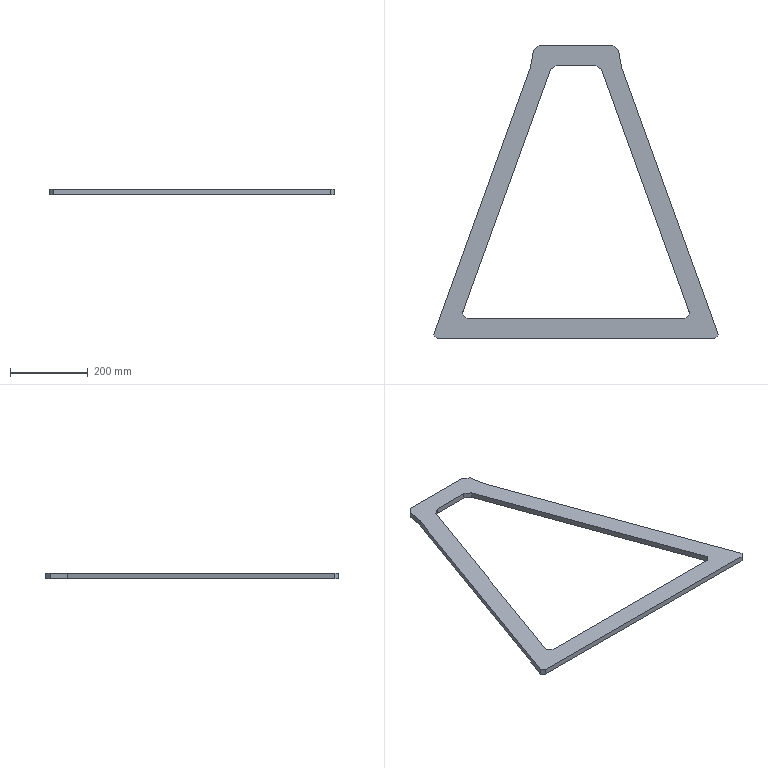Part | SolidWorks | features Extrusion 1 | 1 solid | 20 faces | box 733.425 x 755.65 x 14 mm | volume 1663233 mm3 | plane 20
STEP:
#1=CARTESIAN_POINT('',(-280.465,50.8,0.));
#2=VERTEX_POINT('',#1);
#3=CARTESIAN_POINT('',(280.465,50.8,0.));
#4=VERTEX_POINT('',#3);
#5=CARTESIAN_POINT('',(0.,50.8,0.));
#6=DIRECTION('',(1.,0.,0.));
#7=VECTOR('',#6,1000.);
#8=LINE('',#5,#7);
#9=EDGE_CURVE('',#2,#4,#8,.T.);
#10=ORIENTED_EDGE('',*,*,#9,.F.);
#11=CARTESIAN_POINT('',(-280.465,50.8,14.));
#12=VERTEX_POINT('',#11);
#13=CARTESIAN_POINT('',(-280.465,50.8,14.));
#14=DIRECTION('',(0.,0.,-1.));
#15=VECTOR('',#14,1000.);
#16=LINE('',#13,#15);
#17=EDGE_CURVE('',#12,#2,#16,.T.);
#18=ORIENTED_EDGE('',*,*,#17,.F.);
#19=CARTESIAN_POINT('',(280.465,50.8,14.));
#20=VERTEX_POINT('',#19);
#21=CARTESIAN_POINT('',(0.,50.8,14.));
#22=DIRECTION('',(1.,0.,0.));
#23=VECTOR('',#22,1000.);
#24=LINE('',#21,#23);
#25=EDGE_CURVE('',#12,#20,#24,.T.);
#26=ORIENTED_EDGE('',*,*,#25,.T.);
#27=CARTESIAN_POINT('',(280.465,50.8,14.));
#28=DIRECTION('',(0.,0.,-1.));
#29=VECTOR('',#28,1000.);
#30=LINE('',#27,#29);
#31=EDGE_CURVE('',#20,#4,#30,.T.);
#32=ORIENTED_EDGE('',*,*,#31,.T.);
#33=EDGE_LOOP('',(#10,#18,#26,#32));
#34=FACE_OUTER_BOUND('',#33,.T.);
#35=CARTESIAN_POINT('',(0.,50.8,14.));
#36=DIRECTION('',(0.,1.,0.));
#37=DIRECTION('',(0.,0.,1.));
#38=AXIS2_PLACEMENT_3D('',#35,#36,#37);
#39=PLANE('',#38);
#40=ADVANCED_FACE('',(#34),#39,.T.);
#41=CARTESIAN_POINT('',(-293.165,63.5,0.));
#42=VERTEX_POINT('',#41);
#43=CARTESIAN_POINT('',(-114.833,-114.833,0.));
#44=DIRECTION('',(-0.7071,0.7071,0.));
#45=VECTOR('',#44,1000.);
#46=LINE('',#43,#45);
#47=EDGE_CURVE('',#2,#42,#46,.T.);
#48=ORIENTED_EDGE('',*,*,#47,.T.);
#49=CARTESIAN_POINT('',(-293.165,63.5,14.));
#50=VERTEX_POINT('',#49);
#51=CARTESIAN_POINT('',(-293.165,63.5,14.));
#52=DIRECTION('',(0.,0.,-1.));
#53=VECTOR('',#52,1000.);
#54=LINE('',#51,#53);
#55=EDGE_CURVE('',#50,#42,#54,.T.);
#56=ORIENTED_EDGE('',*,*,#55,.F.);
#57=CARTESIAN_POINT('',(-114.833,-114.833,14.));
#58=DIRECTION('',(-0.7071,0.7071,0.));
#59=VECTOR('',#58,1000.);
#60=LINE('',#57,#59);
#61=EDGE_CURVE('',#12,#50,#60,.T.);
#62=ORIENTED_EDGE('',*,*,#61,.F.);
#63=ORIENTED_EDGE('',*,*,#17,.T.);
#64=EDGE_LOOP('',(#48,#56,#62,#63));
#65=FACE_OUTER_BOUND('',#64,.T.);
#66=CARTESIAN_POINT('',(-114.833,-114.833,14.));
#67=DIRECTION('',(-0.7071,-0.7071,0.));
#68=DIRECTION('',(0.7071,-0.7071,0.));
#69=AXIS2_PLACEMENT_3D('',#66,#67,#68);
#70=PLANE('',#69);
#71=ADVANCED_FACE('',(#65),#70,.F.);
#72=CARTESIAN_POINT('',(-65.476,692.907,0.));
#73=VERTEX_POINT('',#72);
#74=CARTESIAN_POINT('',(-279.553,101.129,0.));
#75=DIRECTION('',(0.3402,0.9404,0.));
#76=VECTOR('',#75,1000.);
#77=LINE('',#74,#76);
#78=EDGE_CURVE('',#42,#73,#77,.T.);
#79=ORIENTED_EDGE('',*,*,#78,.T.);
#80=CARTESIAN_POINT('',(-65.476,692.907,14.));
#81=VERTEX_POINT('',#80);
#82=CARTESIAN_POINT('',(-65.476,692.907,14.));
#83=DIRECTION('',(0.,0.,-1.));
#84=VECTOR('',#83,1000.);
#85=LINE('',#82,#84);
#86=EDGE_CURVE('',#81,#73,#85,.T.);
#87=ORIENTED_EDGE('',*,*,#86,.F.);
#88=CARTESIAN_POINT('',(-279.553,101.129,14.));
#89=DIRECTION('',(0.3402,0.9404,0.));
#90=VECTOR('',#89,1000.);
#91=LINE('',#88,#90);
#92=EDGE_CURVE('',#50,#81,#91,.T.);
#93=ORIENTED_EDGE('',*,*,#92,.F.);
#94=ORIENTED_EDGE('',*,*,#55,.T.);
#95=EDGE_LOOP('',(#79,#87,#93,#94));
#96=FACE_OUTER_BOUND('',#95,.T.);
#97=CARTESIAN_POINT('',(-279.553,101.129,14.));
#98=DIRECTION('',(-0.9404,0.3402,0.));
#99=DIRECTION('',(-0.3402,-0.9404,0.));
#100=AXIS2_PLACEMENT_3D('',#97,#98,#99);
#101=PLANE('',#100);
#102=ADVANCED_FACE('',(#96),#101,.F.);
#103=CARTESIAN_POINT('',(-48.456,704.85,0.));
#104=VERTEX_POINT('',#103);
#105=CARTESIAN_POINT('',(-347.393,495.095,0.));
#106=DIRECTION('',(0.8186,0.5744,0.));
#107=VECTOR('',#106,1000.);
#108=LINE('',#105,#107);
#109=EDGE_CURVE('',#73,#104,#108,.T.);
#110=ORIENTED_EDGE('',*,*,#109,.T.);
#111=CARTESIAN_POINT('',(-48.456,704.85,14.));
#112=VERTEX_POINT('',#111);
#113=CARTESIAN_POINT('',(-48.456,704.85,14.));
#114=DIRECTION('',(0.,0.,-1.));
#115=VECTOR('',#114,1000.);
#116=LINE('',#113,#115);
#117=EDGE_CURVE('',#112,#104,#116,.T.);
#118=ORIENTED_EDGE('',*,*,#117,.F.);
#119=CARTESIAN_POINT('',(-347.393,495.095,14.));
#120=DIRECTION('',(0.8186,0.5744,0.));
#121=VECTOR('',#120,1000.);
#122=LINE('',#119,#121);
#123=EDGE_CURVE('',#81,#112,#122,.T.);
#124=ORIENTED_EDGE('',*,*,#123,.F.);
#125=ORIENTED_EDGE('',*,*,#86,.T.);
#126=EDGE_LOOP('',(#110,#118,#124,#125));
#127=FACE_OUTER_BOUND('',#126,.T.);
#128=CARTESIAN_POINT('',(-347.393,495.095,14.));
#129=DIRECTION('',(-0.5744,0.8186,0.));
#130=DIRECTION('',(-0.8186,-0.5744,0.));
#131=AXIS2_PLACEMENT_3D('',#128,#129,#130);
#132=PLANE('',#131);
#133=ADVANCED_FACE('',(#127),#132,.F.);
#134=CARTESIAN_POINT('',(48.456,704.85,0.));
#135=VERTEX_POINT('',#134);
#136=CARTESIAN_POINT('',(0.,704.85,0.));
#137=DIRECTION('',(-1.,0.,0.));
#138=VECTOR('',#137,1000.);
#139=LINE('',#136,#138);
#140=EDGE_CURVE('',#135,#104,#139,.T.);
#141=ORIENTED_EDGE('',*,*,#140,.F.);
#142=CARTESIAN_POINT('',(48.456,704.85,14.));
#143=VERTEX_POINT('',#142);
#144=CARTESIAN_POINT('',(48.456,704.85,14.));
#145=DIRECTION('',(0.,0.,-1.));
#146=VECTOR('',#145,1000.);
#147=LINE('',#144,#146);
#148=EDGE_CURVE('',#143,#135,#147,.T.);
#149=ORIENTED_EDGE('',*,*,#148,.F.);
#150=CARTESIAN_POINT('',(0.,704.85,14.));
#151=DIRECTION('',(-1.,0.,0.));
#152=VECTOR('',#151,1000.);
#153=LINE('',#150,#152);
#154=EDGE_CURVE('',#143,#112,#153,.T.);
#155=ORIENTED_EDGE('',*,*,#154,.T.);
#156=ORIENTED_EDGE('',*,*,#117,.T.);
#157=EDGE_LOOP('',(#141,#149,#155,#156));
#158=FACE_OUTER_BOUND('',#157,.T.);
#159=CARTESIAN_POINT('',(0.,704.85,14.));
#160=DIRECTION('',(0.,-1.,0.));
#161=DIRECTION('',(0.,0.,-1.));
#162=AXIS2_PLACEMENT_3D('',#159,#160,#161);
#163=PLANE('',#162);
#164=ADVANCED_FACE('',(#158),#163,.T.);
#165=CARTESIAN_POINT('',(65.476,692.907,0.));
#166=VERTEX_POINT('',#165);
#167=CARTESIAN_POINT('',(347.393,495.095,0.));
#168=DIRECTION('',(-0.8186,0.5744,0.));
#169=VECTOR('',#168,1000.);
#170=LINE('',#167,#169);
#171=EDGE_CURVE('',#166,#135,#170,.T.);
#172=ORIENTED_EDGE('',*,*,#171,.F.);
#173=CARTESIAN_POINT('',(65.476,692.907,14.));
#174=VERTEX_POINT('',#173);
#175=CARTESIAN_POINT('',(65.476,692.907,14.));
#176=DIRECTION('',(0.,0.,-1.));
#177=VECTOR('',#176,1000.);
#178=LINE('',#175,#177);
#179=EDGE_CURVE('',#174,#166,#178,.T.);
#180=ORIENTED_EDGE('',*,*,#179,.F.);
#181=CARTESIAN_POINT('',(347.393,495.095,14.));
#182=DIRECTION('',(-0.8186,0.5744,0.));
#183=VECTOR('',#182,1000.);
#184=LINE('',#181,#183);
#185=EDGE_CURVE('',#174,#143,#184,.T.);
#186=ORIENTED_EDGE('',*,*,#185,.T.);
#187=ORIENTED_EDGE('',*,*,#148,.T.);
#188=EDGE_LOOP('',(#172,#180,#186,#187));
#189=FACE_OUTER_BOUND('',#188,.T.);
#190=CARTESIAN_POINT('',(347.393,495.095,14.));
#191=DIRECTION('',(-0.5744,-0.8186,0.));
#192=DIRECTION('',(0.8186,-0.5744,0.));
#193=AXIS2_PLACEMENT_3D('',#190,#191,#192);
#194=PLANE('',#193);
#195=ADVANCED_FACE('',(#189),#194,.T.);
#196=CARTESIAN_POINT('',(293.165,63.5,0.));
#197=VERTEX_POINT('',#196);
#198=CARTESIAN_POINT('',(279.553,101.129,0.));
#199=DIRECTION('',(-0.3402,0.9404,0.));
#200=VECTOR('',#199,1000.);
#201=LINE('',#198,#200);
#202=EDGE_CURVE('',#197,#166,#201,.T.);
#203=ORIENTED_EDGE('',*,*,#202,.F.);
#204=CARTESIAN_POINT('',(293.165,63.5,14.));
#205=VERTEX_POINT('',#204);
#206=CARTESIAN_POINT('',(293.165,63.5,14.));
#207=DIRECTION('',(0.,0.,-1.));
#208=VECTOR('',#207,1000.);
#209=LINE('',#206,#208);
#210=EDGE_CURVE('',#205,#197,#209,.T.);
#211=ORIENTED_EDGE('',*,*,#210,.F.);
#212=CARTESIAN_POINT('',(279.553,101.129,14.));
#213=DIRECTION('',(-0.3402,0.9404,0.));
#214=VECTOR('',#213,1000.);
#215=LINE('',#212,#214);
#216=EDGE_CURVE('',#205,#174,#215,.T.);
#217=ORIENTED_EDGE('',*,*,#216,.T.);
#218=ORIENTED_EDGE('',*,*,#179,.T.);
#219=EDGE_LOOP('',(#203,#211,#217,#218));
#220=FACE_OUTER_BOUND('',#219,.T.);
#221=CARTESIAN_POINT('',(279.553,101.129,14.));
#222=DIRECTION('',(-0.9404,-0.3402,0.));
#223=DIRECTION('',(0.3402,-0.9404,0.));
#224=AXIS2_PLACEMENT_3D('',#221,#222,#223);
#225=PLANE('',#224);
#226=ADVANCED_FACE('',(#220),#225,.T.);
#227=CARTESIAN_POINT('',(-95.25,755.65,0.));
#228=VERTEX_POINT('',#227);
#229=CARTESIAN_POINT('',(95.25,755.65,0.));
#230=VERTEX_POINT('',#229);
#231=CARTESIAN_POINT('',(0.,755.65,0.));
#232=DIRECTION('',(1.,0.,0.));
#233=VECTOR('',#232,1000.);
#234=LINE('',#231,#233);
#235=EDGE_CURVE('',#228,#230,#234,.T.);
#236=ORIENTED_EDGE('',*,*,#235,.F.);
#237=CARTESIAN_POINT('',(-95.25,755.65,14.));
#238=VERTEX_POINT('',#237);
#239=CARTESIAN_POINT('',(-95.25,755.65,14.));
#240=DIRECTION('',(0.,0.,-1.));
#241=VECTOR('',#240,1000.);
#242=LINE('',#239,#241);
#243=EDGE_CURVE('',#238,#228,#242,.T.);
#244=ORIENTED_EDGE('',*,*,#243,.F.);
#245=CARTESIAN_POINT('',(95.25,755.65,14.));
#246=VERTEX_POINT('',#245);
#247=CARTESIAN_POINT('',(0.,755.65,14.));
#248=DIRECTION('',(1.,0.,0.));
#249=VECTOR('',#248,1000.);
#250=LINE('',#247,#249);
#251=EDGE_CURVE('',#238,#246,#250,.T.);
#252=ORIENTED_EDGE('',*,*,#251,.T.);
#253=CARTESIAN_POINT('',(95.25,755.65,14.));
#254=DIRECTION('',(0.,0.,-1.));
#255=VECTOR('',#254,1000.);
#256=LINE('',#253,#255);
#257=EDGE_CURVE('',#246,#230,#256,.T.);
#258=ORIENTED_EDGE('',*,*,#257,.T.);
#259=EDGE_LOOP('',(#236,#244,#252,#258));
#260=FACE_OUTER_BOUND('',#259,.T.);
#261=CARTESIAN_POINT('',(0.,755.65,14.));
#262=DIRECTION('',(0.,1.,0.));
#263=DIRECTION('',(0.,0.,1.));
#264=AXIS2_PLACEMENT_3D('',#261,#262,#263);
#265=PLANE('',#264);
#266=ADVANCED_FACE('',(#260),#265,.T.);
#267=CARTESIAN_POINT('',(-109.538,742.95,0.));
#268=VERTEX_POINT('',#267);
#269=CARTESIAN_POINT('',(-417.261,469.418,0.));
#270=DIRECTION('',(-0.7474,-0.6644,0.));
#271=VECTOR('',#270,1000.);
#272=LINE('',#269,#271);
#273=EDGE_CURVE('',#228,#268,#272,.T.);
#274=ORIENTED_EDGE('',*,*,#273,.T.);
#275=CARTESIAN_POINT('',(-109.538,742.95,14.));
#276=VERTEX_POINT('',#275);
#277=CARTESIAN_POINT('',(-109.538,742.95,14.));
#278=DIRECTION('',(0.,0.,-1.));
#279=VECTOR('',#278,1000.);
#280=LINE('',#277,#279);
#281=EDGE_CURVE('',#276,#268,#280,.T.);
#282=ORIENTED_EDGE('',*,*,#281,.F.);
#283=CARTESIAN_POINT('',(-417.261,469.418,14.));
#284=DIRECTION('',(-0.7474,-0.6644,0.));
#285=VECTOR('',#284,1000.);
#286=LINE('',#283,#285);
#287=EDGE_CURVE('',#238,#276,#286,.T.);
#288=ORIENTED_EDGE('',*,*,#287,.F.);
#289=ORIENTED_EDGE('',*,*,#243,.T.);
#290=EDGE_LOOP('',(#274,#282,#288,#289));
#291=FACE_OUTER_BOUND('',#290,.T.);
#292=CARTESIAN_POINT('',(-417.261,469.418,14.));
#293=DIRECTION('',(0.6644,-0.7474,0.));
#294=DIRECTION('',(0.7474,0.6644,0.));
#295=AXIS2_PLACEMENT_3D('',#292,#293,#294);
#296=PLANE('',#295);
#297=ADVANCED_FACE('',(#291),#296,.F.);
#298=CARTESIAN_POINT('',(-117.475,698.5,0.));
#299=VERTEX_POINT('',#298);
#300=CARTESIAN_POINT('',(-234.722,41.915,0.));
#301=DIRECTION('',(0.1758,0.9844,0.));
#302=VECTOR('',#301,1000.);
#303=LINE('',#300,#302);
#304=EDGE_CURVE('',#299,#268,#303,.T.);
#305=ORIENTED_EDGE('',*,*,#304,.F.);
#306=CARTESIAN_POINT('',(-117.475,698.5,14.));
#307=VERTEX_POINT('',#306);
#308=CARTESIAN_POINT('',(-117.475,698.5,14.));
#309=DIRECTION('',(0.,0.,-1.));
#310=VECTOR('',#309,1000.);
#311=LINE('',#308,#310);
#312=EDGE_CURVE('',#307,#299,#311,.T.);
#313=ORIENTED_EDGE('',*,*,#312,.F.);
#314=CARTESIAN_POINT('',(-234.722,41.915,14.));
#315=DIRECTION('',(0.1758,0.9844,0.));
#316=VECTOR('',#315,1000.);
#317=LINE('',#314,#316);
#318=EDGE_CURVE('',#307,#276,#317,.T.);
#319=ORIENTED_EDGE('',*,*,#318,.T.);
#320=ORIENTED_EDGE('',*,*,#281,.T.);
#321=EDGE_LOOP('',(#305,#313,#319,#320));
#322=FACE_OUTER_BOUND('',#321,.T.);
#323=CARTESIAN_POINT('',(-234.722,41.915,14.));
#324=DIRECTION('',(-0.9844,0.1758,0.));
#325=DIRECTION('',(-0.1758,-0.9844,0.));
#326=AXIS2_PLACEMENT_3D('',#323,#324,#325);
#327=PLANE('',#326);
#328=ADVANCED_FACE('',(#322),#327,.T.);
#329=CARTESIAN_POINT('',(-366.712,9.525,0.));
#330=VERTEX_POINT('',#329);
#331=CARTESIAN_POINT('',(-327.323,118.41,0.));
#332=DIRECTION('',(0.3402,0.9404,0.));
#333=VECTOR('',#332,1000.);
#334=LINE('',#331,#333);
#335=EDGE_CURVE('',#330,#299,#334,.T.);
#336=ORIENTED_EDGE('',*,*,#335,.F.);
#337=CARTESIAN_POINT('',(-366.712,9.525,14.));
#338=VERTEX_POINT('',#337);
#339=CARTESIAN_POINT('',(-366.712,9.525,14.));
#340=DIRECTION('',(0.,0.,-1.));
#341=VECTOR('',#340,1000.);
#342=LINE('',#339,#341);
#343=EDGE_CURVE('',#338,#330,#342,.T.);
#344=ORIENTED_EDGE('',*,*,#343,.F.);
#345=CARTESIAN_POINT('',(-327.323,118.41,14.));
#346=DIRECTION('',(0.3402,0.9404,0.));
#347=VECTOR('',#346,1000.);
#348=LINE('',#345,#347);
#349=EDGE_CURVE('',#338,#307,#348,.T.);
#350=ORIENTED_EDGE('',*,*,#349,.T.);
#351=ORIENTED_EDGE('',*,*,#312,.T.);
#352=EDGE_LOOP('',(#336,#344,#350,#351));
#353=FACE_OUTER_BOUND('',#352,.T.);
#354=CARTESIAN_POINT('',(-327.323,118.41,14.));
#355=DIRECTION('',(-0.9404,0.3402,0.));
#356=DIRECTION('',(-0.3402,-0.9404,0.));
#357=AXIS2_PLACEMENT_3D('',#354,#355,#356);
#358=PLANE('',#357);
#359=ADVANCED_FACE('',(#353),#358,.T.);
#360=CARTESIAN_POINT('',(-357.188,0.,0.));
#361=VERTEX_POINT('',#360);
#362=CARTESIAN_POINT('',(-178.594,-178.594,0.));
#363=DIRECTION('',(-0.7071,0.7071,0.));
#364=VECTOR('',#363,1000.);
#365=LINE('',#362,#364);
#366=EDGE_CURVE('',#361,#330,#365,.T.);
#367=ORIENTED_EDGE('',*,*,#366,.F.);
#368=CARTESIAN_POINT('',(-357.188,0.,14.));
#369=VERTEX_POINT('',#368);
#370=CARTESIAN_POINT('',(-357.188,0.,14.));
#371=DIRECTION('',(0.,0.,-1.));
#372=VECTOR('',#371,1000.);
#373=LINE('',#370,#372);
#374=EDGE_CURVE('',#369,#361,#373,.T.);
#375=ORIENTED_EDGE('',*,*,#374,.F.);
#376=CARTESIAN_POINT('',(-178.594,-178.594,14.));
#377=DIRECTION('',(-0.7071,0.7071,0.));
#378=VECTOR('',#377,1000.);
#379=LINE('',#376,#378);
#380=EDGE_CURVE('',#369,#338,#379,.T.);
#381=ORIENTED_EDGE('',*,*,#380,.T.);
#382=ORIENTED_EDGE('',*,*,#343,.T.);
#383=EDGE_LOOP('',(#367,#375,#381,#382));
#384=FACE_OUTER_BOUND('',#383,.T.);
#385=CARTESIAN_POINT('',(-178.594,-178.594,14.));
#386=DIRECTION('',(-0.7071,-0.7071,0.));
#387=DIRECTION('',(0.7071,-0.7071,0.));
#388=AXIS2_PLACEMENT_3D('',#385,#386,#387);
#389=PLANE('',#388);
#390=ADVANCED_FACE('',(#384),#389,.T.);
#391=CARTESIAN_POINT('',(357.188,0.,0.));
#392=VERTEX_POINT('',#391);
#393=CARTESIAN_POINT('',(0.,0.,0.));
#394=DIRECTION('',(-1.,0.,0.));
#395=VECTOR('',#394,1000.);
#396=LINE('',#393,#395);
#397=EDGE_CURVE('',#392,#361,#396,.T.);
#398=ORIENTED_EDGE('',*,*,#397,.F.);
#399=CARTESIAN_POINT('',(357.188,0.,14.));
#400=VERTEX_POINT('',#399);
#401=CARTESIAN_POINT('',(357.188,0.,14.));
#402=DIRECTION('',(0.,0.,-1.));
#403=VECTOR('',#402,1000.);
#404=LINE('',#401,#403);
#405=EDGE_CURVE('',#400,#392,#404,.T.);
#406=ORIENTED_EDGE('',*,*,#405,.F.);
#407=CARTESIAN_POINT('',(0.,0.,14.));
#408=DIRECTION('',(-1.,0.,0.));
#409=VECTOR('',#408,1000.);
#410=LINE('',#407,#409);
#411=EDGE_CURVE('',#400,#369,#410,.T.);
#412=ORIENTED_EDGE('',*,*,#411,.T.);
#413=ORIENTED_EDGE('',*,*,#374,.T.);
#414=EDGE_LOOP('',(#398,#406,#412,#413));
#415=FACE_OUTER_BOUND('',#414,.T.);
#416=CARTESIAN_POINT('',(0.,0.,14.));
#417=DIRECTION('',(0.,-1.,0.));
#418=DIRECTION('',(1.,0.,0.));
#419=AXIS2_PLACEMENT_3D('',#416,#417,#418);
#420=PLANE('',#419);
#421=ADVANCED_FACE('',(#415),#420,.T.);
#422=CARTESIAN_POINT('',(366.713,9.525,0.));
#423=VERTEX_POINT('',#422);
#424=CARTESIAN_POINT('',(178.594,-178.594,0.));
#425=DIRECTION('',(0.7071,0.7071,0.));
#426=VECTOR('',#425,1000.);
#427=LINE('',#424,#426);
#428=EDGE_CURVE('',#392,#423,#427,.T.);
#429=ORIENTED_EDGE('',*,*,#428,.T.);
#430=CARTESIAN_POINT('',(366.713,9.525,14.));
#431=VERTEX_POINT('',#430);
#432=CARTESIAN_POINT('',(366.713,9.525,14.));
#433=DIRECTION('',(0.,0.,-1.));
#434=VECTOR('',#433,1000.);
#435=LINE('',#432,#434);
#436=EDGE_CURVE('',#431,#423,#435,.T.);
#437=ORIENTED_EDGE('',*,*,#436,.F.);
#438=CARTESIAN_POINT('',(178.594,-178.594,14.));
#439=DIRECTION('',(0.7071,0.7071,0.));
#440=VECTOR('',#439,1000.);
#441=LINE('',#438,#440);
#442=EDGE_CURVE('',#400,#431,#441,.T.);
#443=ORIENTED_EDGE('',*,*,#442,.F.);
#444=ORIENTED_EDGE('',*,*,#405,.T.);
#445=EDGE_LOOP('',(#429,#437,#443,#444));
#446=FACE_OUTER_BOUND('',#445,.T.);
#447=CARTESIAN_POINT('',(178.594,-178.594,14.));
#448=DIRECTION('',(-0.7071,0.7071,0.));
#449=DIRECTION('',(-0.7071,-0.7071,0.));
#450=AXIS2_PLACEMENT_3D('',#447,#448,#449);
#451=PLANE('',#450);
#452=ADVANCED_FACE('',(#446),#451,.F.);
#453=CARTESIAN_POINT('',(117.475,698.5,0.));
#454=VERTEX_POINT('',#453);
#455=CARTESIAN_POINT('',(327.323,118.41,0.));
#456=DIRECTION('',(-0.3402,0.9404,0.));
#457=VECTOR('',#456,1000.);
#458=LINE('',#455,#457);
#459=EDGE_CURVE('',#423,#454,#458,.T.);
#460=ORIENTED_EDGE('',*,*,#459,.T.);
#461=CARTESIAN_POINT('',(117.475,698.5,14.));
#462=VERTEX_POINT('',#461);
#463=CARTESIAN_POINT('',(117.475,698.5,14.));
#464=DIRECTION('',(0.,0.,-1.));
#465=VECTOR('',#464,1000.);
#466=LINE('',#463,#465);
#467=EDGE_CURVE('',#462,#454,#466,.T.);
#468=ORIENTED_EDGE('',*,*,#467,.F.);
#469=CARTESIAN_POINT('',(327.323,118.41,14.));
#470=DIRECTION('',(-0.3402,0.9404,0.));
#471=VECTOR('',#470,1000.);
#472=LINE('',#469,#471);
#473=EDGE_CURVE('',#431,#462,#472,.T.);
#474=ORIENTED_EDGE('',*,*,#473,.F.);
#475=ORIENTED_EDGE('',*,*,#436,.T.);
#476=EDGE_LOOP('',(#460,#468,#474,#475));
#477=FACE_OUTER_BOUND('',#476,.T.);
#478=CARTESIAN_POINT('',(327.323,118.41,14.));
#479=DIRECTION('',(-0.9404,-0.3402,0.));
#480=DIRECTION('',(0.3402,-0.9404,0.));
#481=AXIS2_PLACEMENT_3D('',#478,#479,#480);
#482=PLANE('',#481);
#483=ADVANCED_FACE('',(#477),#482,.F.);
#484=CARTESIAN_POINT('',(109.538,742.95,0.));
#485=VERTEX_POINT('',#484);
#486=CARTESIAN_POINT('',(234.722,41.915,0.));
#487=DIRECTION('',(-0.1758,0.9844,0.));
#488=VECTOR('',#487,1000.);
#489=LINE('',#486,#488);
#490=EDGE_CURVE('',#454,#485,#489,.T.);
#491=ORIENTED_EDGE('',*,*,#490,.T.);
#492=CARTESIAN_POINT('',(109.538,742.95,14.));
#493=VERTEX_POINT('',#492);
#494=CARTESIAN_POINT('',(109.538,742.95,14.));
#495=DIRECTION('',(0.,0.,-1.));
#496=VECTOR('',#495,1000.);
#497=LINE('',#494,#496);
#498=EDGE_CURVE('',#493,#485,#497,.T.);
#499=ORIENTED_EDGE('',*,*,#498,.F.);
#500=CARTESIAN_POINT('',(234.722,41.915,14.));
#501=DIRECTION('',(-0.1758,0.9844,0.));
#502=VECTOR('',#501,1000.);
#503=LINE('',#500,#502);
#504=EDGE_CURVE('',#462,#493,#503,.T.);
#505=ORIENTED_EDGE('',*,*,#504,.F.);
#506=ORIENTED_EDGE('',*,*,#467,.T.);
#507=EDGE_LOOP('',(#491,#499,#505,#506));
#508=FACE_OUTER_BOUND('',#507,.T.);
#509=CARTESIAN_POINT('',(234.722,41.915,14.));
#510=DIRECTION('',(-0.9844,-0.1758,0.));
#511=DIRECTION('',(0.1758,-0.9844,0.));
#512=AXIS2_PLACEMENT_3D('',#509,#510,#511);
#513=PLANE('',#512);
#514=ADVANCED_FACE('',(#508),#513,.F.);
#515=CARTESIAN_POINT('',(417.261,469.418,0.));
#516=DIRECTION('',(0.7474,-0.6644,0.));
#517=VECTOR('',#516,1000.);
#518=LINE('',#515,#517);
#519=EDGE_CURVE('',#230,#485,#518,.T.);
#520=ORIENTED_EDGE('',*,*,#519,.F.);
#521=ORIENTED_EDGE('',*,*,#257,.F.);
#522=CARTESIAN_POINT('',(417.261,469.418,14.));
#523=DIRECTION('',(0.7474,-0.6644,0.));
#524=VECTOR('',#523,1000.);
#525=LINE('',#522,#524);
#526=EDGE_CURVE('',#246,#493,#525,.T.);
#527=ORIENTED_EDGE('',*,*,#526,.T.);
#528=ORIENTED_EDGE('',*,*,#498,.T.);
#529=EDGE_LOOP('',(#520,#521,#527,#528));
#530=FACE_OUTER_BOUND('',#529,.T.);
#531=CARTESIAN_POINT('',(417.261,469.418,14.));
#532=DIRECTION('',(0.6644,0.7474,0.));
#533=DIRECTION('',(-0.7474,0.6644,0.));
#534=AXIS2_PLACEMENT_3D('',#531,#532,#533);
#535=PLANE('',#534);
#536=ADVANCED_FACE('',(#530),#535,.T.);
#537=CARTESIAN_POINT('',(114.833,-114.833,0.));
#538=DIRECTION('',(0.7071,0.7071,0.));
#539=VECTOR('',#538,1000.);
#540=LINE('',#537,#539);
#541=EDGE_CURVE('',#4,#197,#540,.T.);
#542=ORIENTED_EDGE('',*,*,#541,.F.);
#543=ORIENTED_EDGE('',*,*,#31,.F.);
#544=CARTESIAN_POINT('',(114.833,-114.833,14.));
#545=DIRECTION('',(0.7071,0.7071,0.));
#546=VECTOR('',#545,1000.);
#547=LINE('',#544,#546);
#548=EDGE_CURVE('',#20,#205,#547,.T.);
#549=ORIENTED_EDGE('',*,*,#548,.T.);
#550=ORIENTED_EDGE('',*,*,#210,.T.);
#551=EDGE_LOOP('',(#542,#543,#549,#550));
#552=FACE_OUTER_BOUND('',#551,.T.);
#553=CARTESIAN_POINT('',(114.833,-114.833,14.));
#554=DIRECTION('',(-0.7071,0.7071,0.));
#555=DIRECTION('',(-0.7071,-0.7071,0.));
#556=AXIS2_PLACEMENT_3D('',#553,#554,#555);
#557=PLANE('',#556);
#558=ADVANCED_FACE('',(#552),#557,.T.);
#559=ORIENTED_EDGE('',*,*,#251,.F.);
#560=ORIENTED_EDGE('',*,*,#287,.T.);
#561=ORIENTED_EDGE('',*,*,#318,.F.);
#562=ORIENTED_EDGE('',*,*,#349,.F.);
#563=ORIENTED_EDGE('',*,*,#380,.F.);
#564=ORIENTED_EDGE('',*,*,#411,.F.);
#565=ORIENTED_EDGE('',*,*,#442,.T.);
#566=ORIENTED_EDGE('',*,*,#473,.T.);
#567=ORIENTED_EDGE('',*,*,#504,.T.);
#568=ORIENTED_EDGE('',*,*,#526,.F.);
#569=EDGE_LOOP('',(#559,#560,#561,#562,#563,#564,#565,#566,#567,#568));
#570=FACE_OUTER_BOUND('',#569,.T.);
#571=ORIENTED_EDGE('',*,*,#25,.F.);
#572=ORIENTED_EDGE('',*,*,#61,.T.);
#573=ORIENTED_EDGE('',*,*,#92,.T.);
#574=ORIENTED_EDGE('',*,*,#123,.T.);
#575=ORIENTED_EDGE('',*,*,#154,.F.);
#576=ORIENTED_EDGE('',*,*,#185,.F.);
#577=ORIENTED_EDGE('',*,*,#216,.F.);
#578=ORIENTED_EDGE('',*,*,#548,.F.);
#579=EDGE_LOOP('',(#571,#572,#573,#574,#575,#576,#577,#578));
#580=FACE_BOUND('',#579,.T.);
#581=CARTESIAN_POINT('',(0.,0.,14.));
#582=DIRECTION('',(0.,0.,1.));
#583=DIRECTION('',(1.,0.,0.));
#584=AXIS2_PLACEMENT_3D('',#581,#582,#583);
#585=PLANE('',#584);
#586=ADVANCED_FACE('',(#570,#580),#585,.T.);
#587=ORIENTED_EDGE('',*,*,#235,.T.);
#588=ORIENTED_EDGE('',*,*,#519,.T.);
#589=ORIENTED_EDGE('',*,*,#490,.F.);
#590=ORIENTED_EDGE('',*,*,#459,.F.);
#591=ORIENTED_EDGE('',*,*,#428,.F.);
#592=ORIENTED_EDGE('',*,*,#397,.T.);
#593=ORIENTED_EDGE('',*,*,#366,.T.);
#594=ORIENTED_EDGE('',*,*,#335,.T.);
#595=ORIENTED_EDGE('',*,*,#304,.T.);
#596=ORIENTED_EDGE('',*,*,#273,.F.);
#597=EDGE_LOOP('',(#587,#588,#589,#590,#591,#592,#593,#594,#595,#596));
#598=FACE_OUTER_BOUND('',#597,.T.);
#599=ORIENTED_EDGE('',*,*,#9,.T.);
#600=ORIENTED_EDGE('',*,*,#541,.T.);
#601=ORIENTED_EDGE('',*,*,#202,.T.);
#602=ORIENTED_EDGE('',*,*,#171,.T.);
#603=ORIENTED_EDGE('',*,*,#140,.T.);
#604=ORIENTED_EDGE('',*,*,#109,.F.);
#605=ORIENTED_EDGE('',*,*,#78,.F.);
#606=ORIENTED_EDGE('',*,*,#47,.F.);
#607=EDGE_LOOP('',(#599,#600,#601,#602,#603,#604,#605,#606));
#608=FACE_BOUND('',#607,.T.);
#609=CARTESIAN_POINT('',(0.,0.,0.));
#610=DIRECTION('',(0.,0.,1.));
#611=DIRECTION('',(1.,0.,0.));
#612=AXIS2_PLACEMENT_3D('',#609,#610,#611);
#613=PLANE('',#612);
#614=ADVANCED_FACE('',(#598,#608),#613,.F.);
#615=CLOSED_SHELL('',(#40,#71,#102,#133,#164,#195,#226,#266,#297,#328,#359,#390,#421,#452,#483,#514,#536,#558,#586,#614));
#616=MANIFOLD_SOLID_BREP('',#615);
#617=CARTESIAN_POINT('',(0.,0.,0.));
#618=DIRECTION('',(0.,0.,1.));
#619=DIRECTION('',(1.,0.,0.));
#620=AXIS2_PLACEMENT_3D('',#617,#618,#619);
#621=(LENGTH_UNIT()NAMED_UNIT(*)SI_UNIT(.MILLI.,.METRE.));
#622=UNCERTAINTY_MEASURE_WITH_UNIT(LENGTH_MEASURE(0.00001),#621,'','');
#623=(NAMED_UNIT(*)PLANE_ANGLE_UNIT()SI_UNIT($,.RADIAN.));
#624=(NAMED_UNIT(*)SI_UNIT($,.STERADIAN.)SOLID_ANGLE_UNIT());
#625=(GEOMETRIC_REPRESENTATION_CONTEXT(3)GLOBAL_UNCERTAINTY_ASSIGNED_CONTEXT((#622))GLOBAL_UNIT_ASSIGNED_CONTEXT((#621,#623,#624))REPRESENTATION_CONTEXT('',''));
#626=ADVANCED_BREP_SHAPE_REPRESENTATION('',(#616,#620),#625);